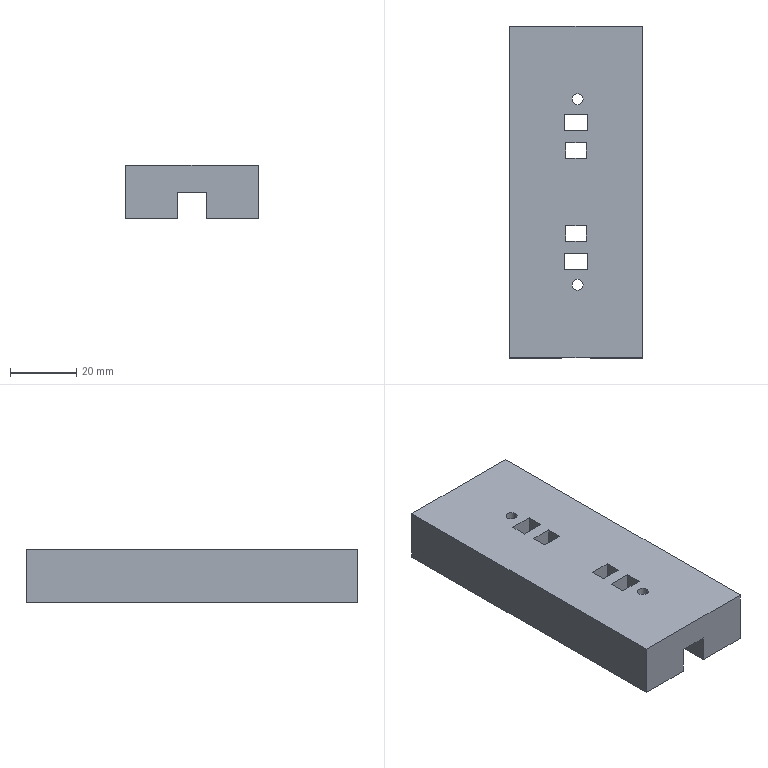Part | STEP file | Riveting upper die seat | 1 solid | 46 faces | box 40 x 100 x 16 mm | volume 55230 mm3 | plane 26 | cylinder 12 | cone 8 | commonest cylinder face diameters 4.2 x8 3.3 x4